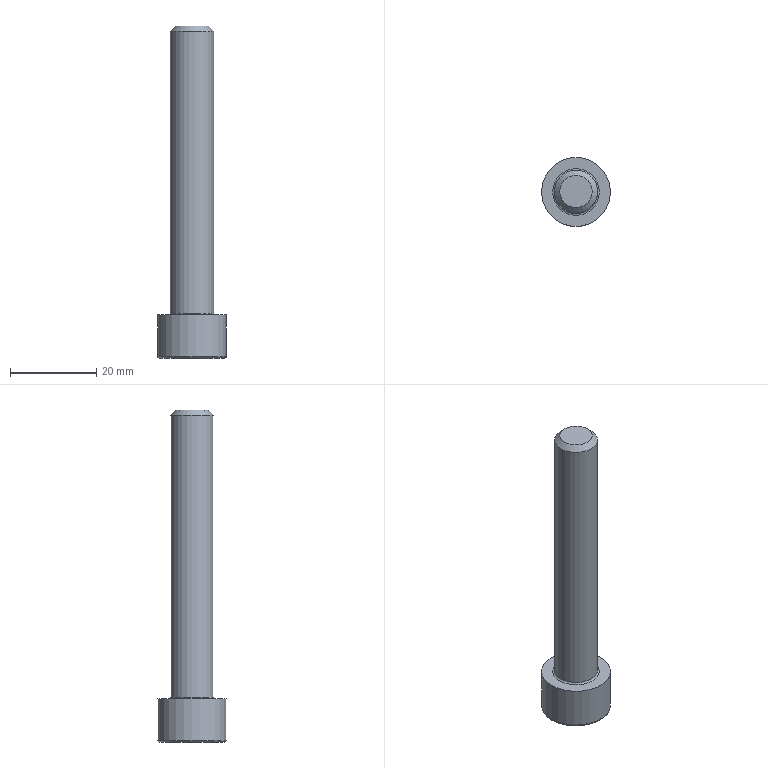Part | STEP file | solid 167 | 1 solid | 15 faces | box 16 x 16 x 77 mm | volume 6973 mm3 | plane 10 | cylinder 2 | torus 2 | cone 1 | commonest cylinder face diameters 10 x1 16 x1